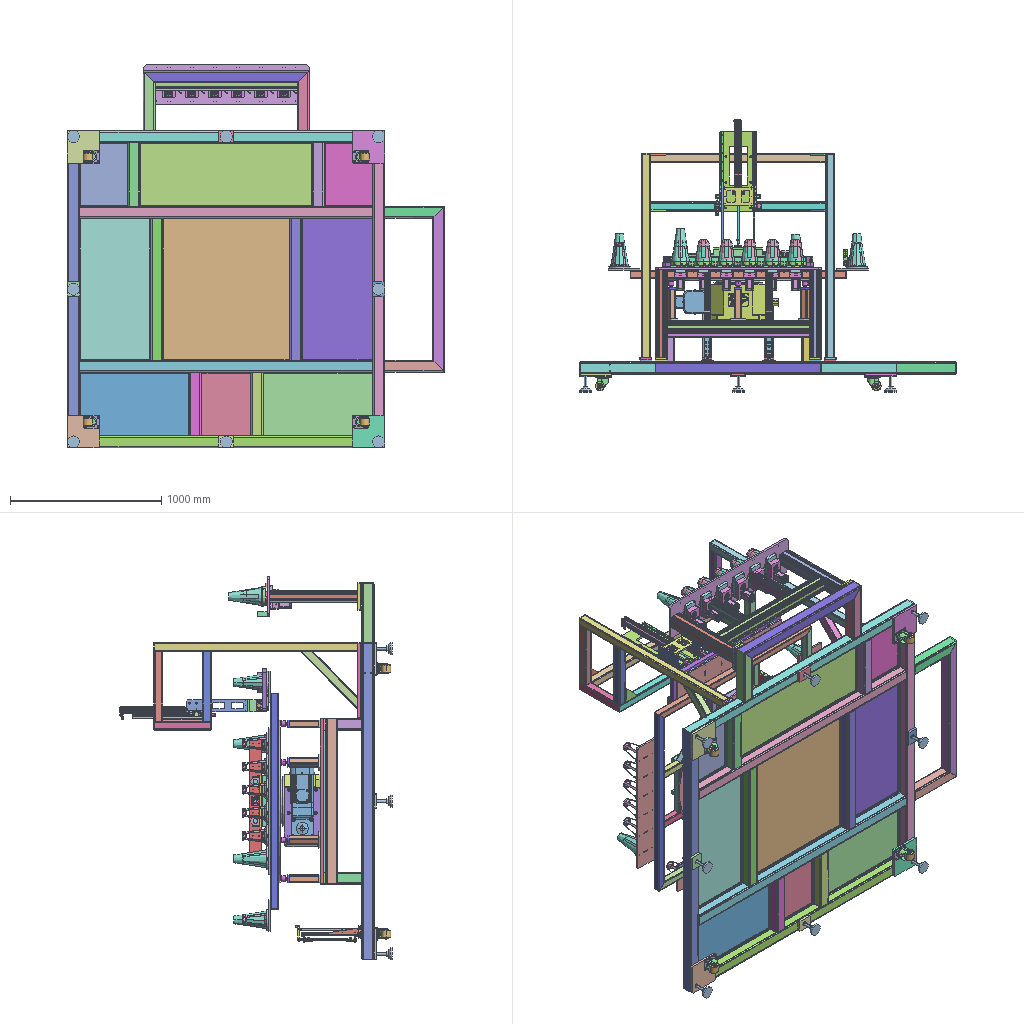Assembly | SolidWorks | 142 different items | 599 placed | box 2495 x 1802 x 2540 mm
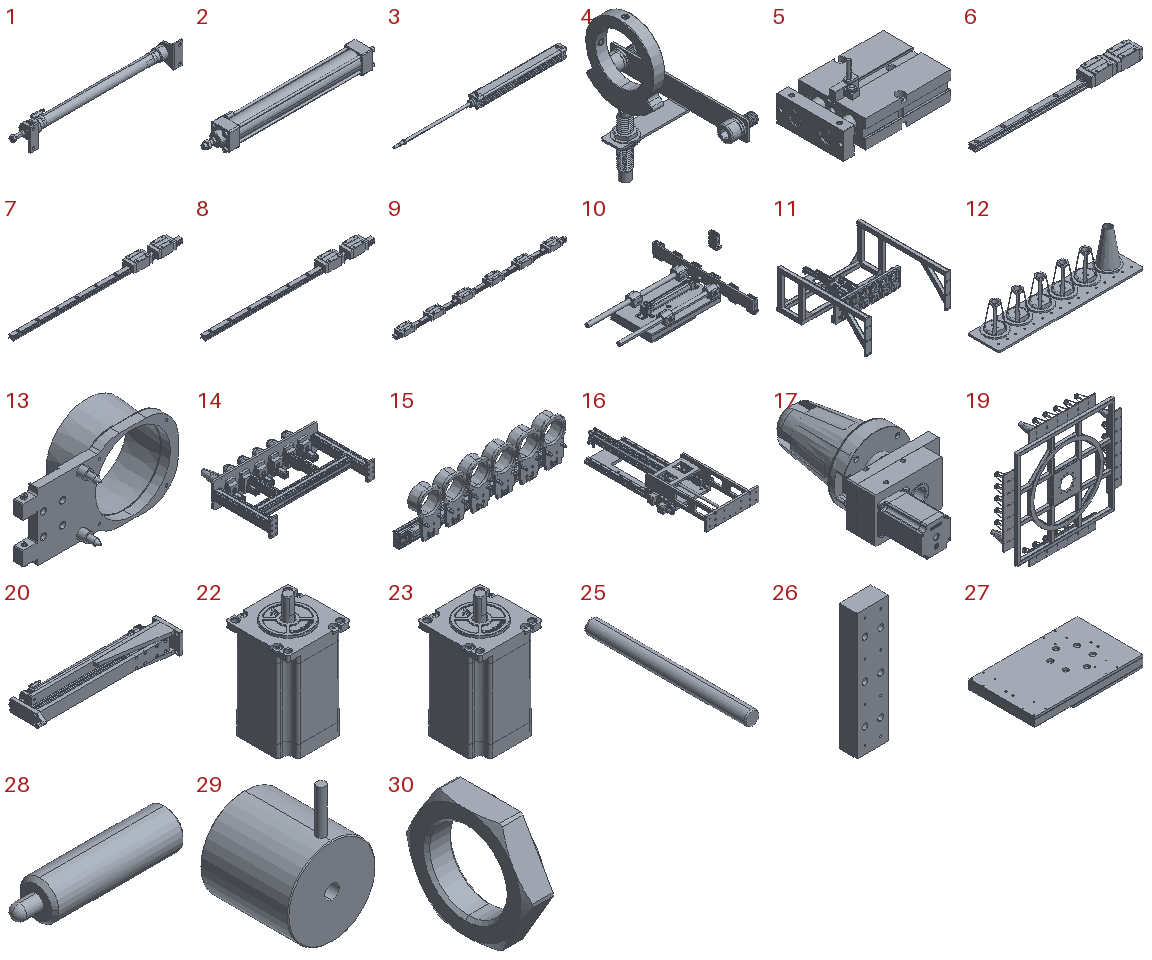Parts list (item | name | quantity | parent item | size | volume | features):
1 | (subassembly) | x2 | in 20 | 392 x 41.5 x 54 mm | 88963 mm3 | -
2 | (subassembly) | x1 | in 10 | 451 x 53.518 x 51.2 mm | 402032 mm3 | -
3 | (subassembly) | x1 | in 16 | 845 x 46.8 x 46.5 mm | 590487 mm3 | -
4 | (subassembly) | x1 | in 24 | 87 x 140.21 x 144 mm | 53103 mm3 | -
5 | (subassembly) | x7 | in 10 | 98 x 62 x 48 mm | 117635 mm3 | -
6 | (subassembly) | x2 | in 20 | 380 x 34 x 28 mm | 139107 mm3 | -
7 | (subassembly) | x1 | in 16 | 520 x 34 x 28 mm | 162854 mm3 | -
8 | (subassembly) | x1 | in 16 | 520 x 34 x 28 mm | 162854 mm3 | -
9 | (subassembly) | x1 | in 15 | 930 x 44 x 30 mm | 645154 mm3 | -
10 | (subassembly) | x1 | in 21 | - | 9355579 mm3 | -
11 | (subassembly) | x1 | in 21 | - | 24248419 mm3 | -
12 | (subassembly) | x4 | in 19 | 975 x 210 x 240 mm | 4305889 mm3 | -
13 | (subassembly) | x6 | in 15 | 257 x 108 x 135 mm | 263904 mm3 | -
14 | (subassembly) | x1 | in 18 | - | 19249167 mm3 | -
15 | (subassembly) | x1 | in 11 | 985 x 114 x 267 mm | 3601226 mm3 | -
16 | (subassembly) | x1 | in 11 | 320 x 857.77 x 130.25 mm | 3607069 mm3 | -
17 | (subassembly) | x6 | in 14 | - | 1851782 mm3 | -
18 | (subassembly) | x1 | in 21 | - | - | -
19 | (subassembly) | x1 | in 21 | - | 27946605 mm3 | -
20 | (subassembly) | x2 | in 21 | 429 x 109.5 x 60 mm | 759599 mm3 | -
21 | (subassembly) | x1 | - | - | - | -
22 | (subassembly) | x6 | in 17 | 56.538 x 56.538 x 106 mm | 169179 mm3 | -
23 | (subassembly) | x6 | in 22 | 56.538 x 56.538 x 106 mm | 169179 mm3 | -
24 | (subassembly) | x1 | in 18 | - | - | -
25 | - | x6 | in 23 | 8 x 92 x 8 mm | 4599 mm3 | features BaseBody 1
26 | - | x1 | in 11 | 80 x 45 x 320 mm | 1113853 mm3 | features BaseBody 1
27 | - | x1 | in 10 | 560 x 340 x 60 mm | 3618040 mm3 | features BaseBody 7
28 | - | x12 | in 13 | 32 x 8 x 8 mm | 1371 mm3 | features BaseBody 1
29 | - | x24 | in 17 | 20 x 20 x 30 mm | 6254 mm3 | features BaseBody 1
30 | - | x4 | in 1 | 7 x 33 x 29 mm | 2695 mm3 | features BaseBody 1
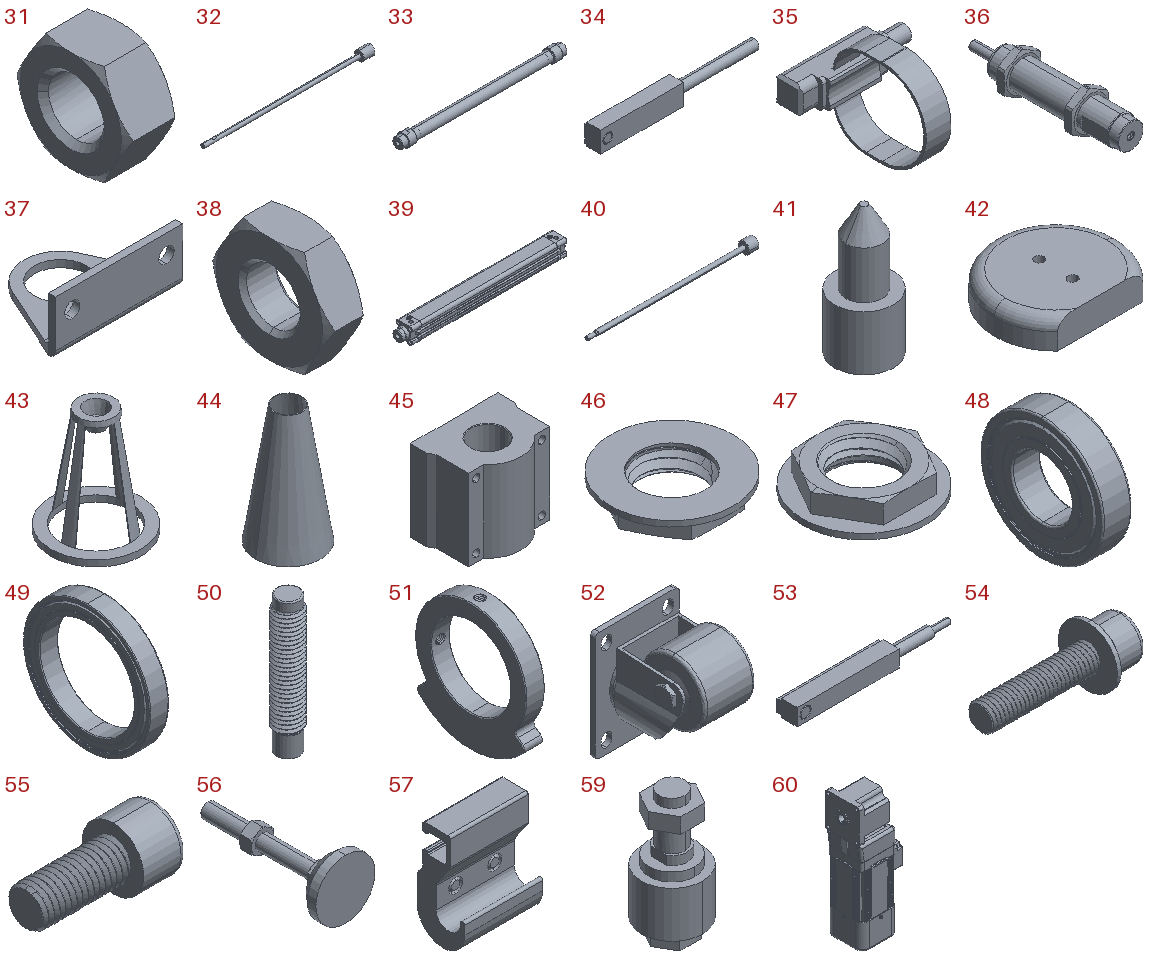31 | - | x2 | in 1 | 6 x 13.856 x 12.001 mm | 526.097 mm3 | features BaseBody 1
32 | - | x2 | in 1 | 339 x 19.5 x 19.5 mm | 22445 mm3 | features BaseBody 1
33 | - | x2 | in 1 | 350 x 27 x 27 mm | 44687 mm3 | features BaseBody 1
34 | - | x1 | in 3 | 48.8 x 5.6 x 6.3 mm | 899.301 mm3 | features BaseBody 1
35 | - | x4 | in 1 | 30 x 30.9 x 22.4 mm | 1513 mm3 | features BaseBody 1
36 | - | x1 | in 16 | 26 x 112.5 x 29.132 mm | 32268 mm3 | features BaseBody 3
37 | - | x4 | in 1 | 54 x 40.5 x 23 mm | 6445 mm3 | features BaseBody 1
38 | - | x1 | in 3 | 6 x 19.63 x 17 mm | 1126 mm3 | features BaseBody 1
39 | - | x1 | in 3 | 466 x 46.5 x 46.5 mm | 520717 mm3 | features BaseBody 1
40 | - | x1 | in 3 | 458 x 31.1 x 31.1 mm | 67743 mm3 | features BaseBody 1
41 | - | x12 | in 13 | 16 x 16 x 35 mm | 4084 mm3 | features BaseBody 1
42 | - | x24 | in 12 | 111 x 95.5 x 25 mm | 213112 mm3 | features BaseBody 1
43 | - | x24 | in 12 | 144 x 144 x 170 mm | 89081 mm3 | features BaseBody 2
44 | - | x5 | in 12, 14 | 120 x 120 x 218 mm | 58583 mm3 | features BaseBody 1
45 | - | x4 | in 10 | 78 x 59.5 x 72 mm | 226738 mm3 | features BaseBody 1
46 | - | x1 | in 4 | 22 x 22 x 4.5 mm | 732.317 mm3 | features BaseBody 1
47 | - | x1 | in 4 | 22 x 22 x 4.5 mm | 732.33 mm3 | features BaseBody 1
48 | - | x6 | in 17 | 17 x 72 x 72 mm | 43583 mm3 | features BaseBody 1
49 | - | x6 | in 17 | 7 x 47 x 47 mm | 4480 mm3 | features BaseBody 1
50 | - | x1 | in 4 | 12 x 12 x 62 mm | 5810 mm3 | features BaseBody 1
51 | - | x1 | in 4 | 12 x 70 x 80 mm | 30669 mm3 | features BaseBody 1
52 | - | x4 | in 18 | 82 x 96 x 111.5 mm | 252248 mm3 | features BaseBody 3
53 | - | x2 | in 2 | 41.8 x 5.7 x 4.4 mm | 661.389 mm3 | features BaseBody 1
54 | - | x4 | in 24 | 53.5 x 22 x 22 mm | 5383 mm3 | features BaseBody 1
55 | - | x4 | in 24 | 40 x 19 x 19 mm | 5409 mm3 | features BaseBody 1
56 | - | x8 | in 18 | 80 x 187 x 80 mm | 168860 mm3 | features BaseBody 2
57 | - | x2 | in 2 | 18 x 12.6 x 23 mm | 2035 mm3 | features BaseBody 1
58 | - | x1 | in 24 | - | - | features BaseBody 1
59 | - | x1 | in 10 | 28 x 28 x 58 mm | 19476 mm3 | features BaseBody 1
60 | - | x1 | in 24 | 220.628 x 166 x 541 mm | 11207085 mm3 | features BaseBody 1
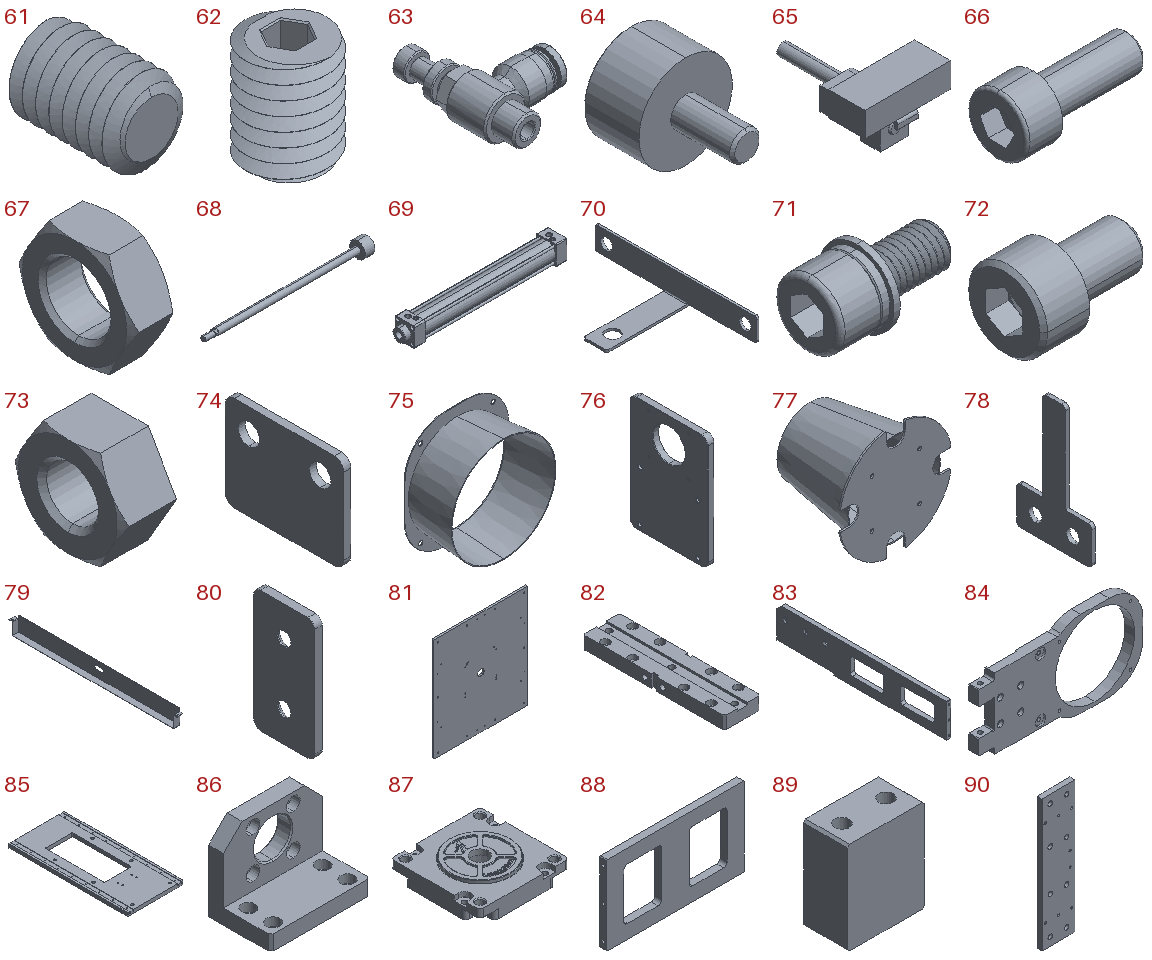61 | - | x1 | in 4 | 6 x 8 x 6 mm | 142.48 mm3 | features BaseBody 1
62 | - | x1 | in 4 | 6 x 6 x 8 mm | 142.472 mm3 | features BaseBody 1
63 | - | x1 | in 16 | 30 x 41.5 x 14 mm | 4765 mm3 | features BaseBody 1
64 | - | x6 | in 18 | 38 x 57 x 38 mm | 31976 mm3 | features BaseBody 1
65 | - | x7 | in 5 | 21 x 26 x 14 mm | 1685 mm3 | features BaseBody 1
66 | - | x4 | in 2 | 22 x 10 x 10 mm | 853.723 mm3 | features BaseBody 1
67 | - | x1 | in 2 | 7 x 19.63 x 17 mm | 1102 mm3 | features BaseBody 1
68 | - | x1 | in 2 | 407.5 x 39.5 x 39.5 mm | 104182 mm3 | features BaseBody 1
69 | - | x1 | in 2 | 408 x 50 x 50 mm | 287943 mm3 | features BaseBody 1
70 | - | x1 | in 4 | 72 x 140.21 x 22 mm | 7925 mm3 | features BaseBody 1
71 | - | x2 | in 4 | 30.5 x 18 x 18 mm | 3479 mm3 | features BaseBody 1
72 | - | x6 | in 13 | 13 x 8.5 x 8.5 mm | 397.23 mm3 | features BaseBody 1
73 | - | x6 | in 18 | 10 x 21.939 x 19 mm | 2287 mm3 | features BaseBody 1
74 | - | x2 | in 16 | 1.5 x 25 x 20 mm | 697.137 mm3 | features BaseBody 1
75 | - | x6 | in 13 | 135 x 61 x 150 mm | 30112 mm3 | features BaseBody 2
76 | - | x1 | in 24 | 20 x 240 x 350 mm | 1488667 mm3 | features BaseBody 1
77 | - | x6 | in 17 | 131.373 x 102 x 131.373 mm | 54164 mm3 | features BaseBody 2
78 | - | x6 | in 17 | 1 x 20 x 34 mm | 323.47 mm3 | features BaseBody 1
79 | - | x1 | in 14 | 35 x 938 x 82 mm | 107925 mm3 | features BaseBody 1
80 | - | x2 | in 15 | 5 x 40 x 80 mm | 14588 mm3 | features BaseBody 1
81 | - | x1 | in 18 | 1000 x 20 x 1100 mm | 21854626 mm3 | features BaseBody 1
82 | - | x2 | in 16 | 35 x 135 x 12 mm | 47871 mm3 | features BaseBody 1
83 | - | x2 | in 16 | 10 x 405 x 80 mm | 250680 mm3 | features BaseBody 1
84 | - | x6 | in 13 | 257 x 15 x 134 mm | 222484 mm3 | features BaseBody 1
85 | - | x1 | in 16 | 245 x 524 x 15 mm | 1411431 mm3 | features BaseBody 1
86 | - | x1 | in 16 | 80 x 50 x 65 mm | 80960 mm3 | features BaseBody 1
87 | - | x6 | in 23 | 56.4 x 56.4 x 13.3 mm | 19484 mm3 | features BaseBody 1
88 | - | x1 | in 16 | 200 x 10 x 115 mm | 146843 mm3 | features BaseBody 1
89 | - | x6 | in 15 | 35 x 20 x 42 mm | 25659 mm3 | features BaseBody 1
90 | - | x1 | in 16 | 80 x 12 x 320 mm | 296552 mm3 | features BaseBody 1
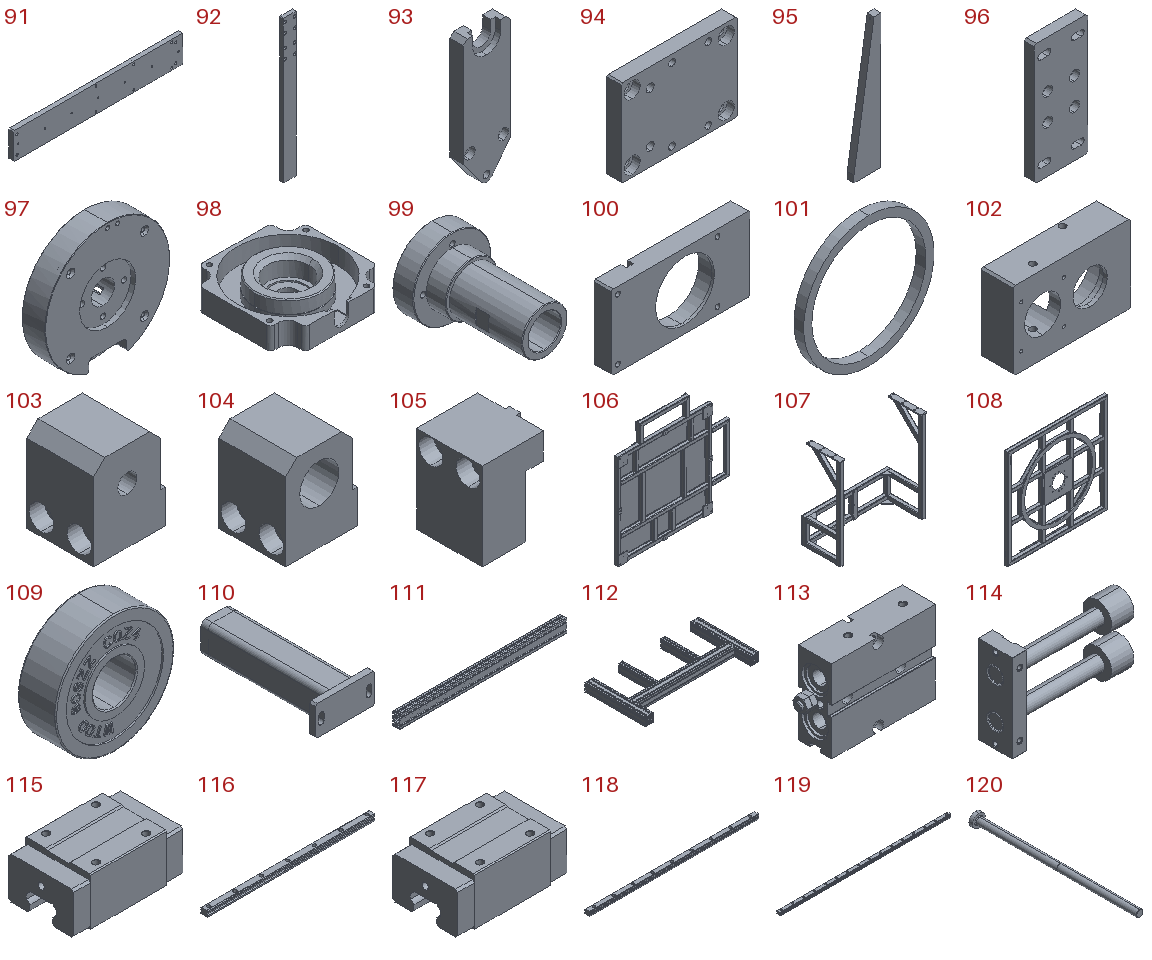91 | - | x2 | in 20 | 380 x 10 x 60 mm | 224318 mm3 | features BaseBody 1
92 | - | x2 | in 20 | 35 x 10 x 380 mm | 129960 mm3 | features BaseBody 1
93 | - | x2 | in 20 | 35 x 10 x 100 mm | 28731 mm3 | features BaseBody 1
94 | - | x2 | in 20 | 80 x 10 x 60 mm | 43027 mm3 | features BaseBody 1
95 | - | x4 | in 20 | 40 x 10 x 200 mm | 51054 mm3 | features BaseBody 1
96 | - | x2 | in 14 | 80 x 15 x 180 mm | 198624 mm3 | features BaseBody 1
97 | - | x6 | in 17 | 134 x 25 x 134 mm | 280686 mm3 | features BaseBody 1
98 | - | x6 | in 23 | - | - | features RefSurface 4, BaseBody 1
99 | - | x6 | in 17 | 60 x 87 x 60 mm | 74210 mm3 | features BaseBody 1
100 | - | x6 | in 17 | 160 x 20 x 86 mm | 181258 mm3 | features BaseBody 1
101 | - | x12 | in 17 | 40 x 3 x 40 mm | 883.573 mm3 | features BaseBody 1
102 | - | x6 | in 17 | 130 x 35.485 x 86 mm | 236354 mm3 | features BaseBody 1
103 | - | x1 | in 16 | 34 x 30 x 40 mm | 31581 mm3 | features BaseBody 1
104 | - | x1 | in 16 | 34 x 30 x 40 mm | 26067 mm3 | features BaseBody 1
105 | - | x2 | in 16 | 30 x 30 x 40 mm | 24257 mm3 | features BaseBody 1
106 | - | x1 | in 18 | 2495 x 350 x 2495 mm | 50017538 mm3 | features BaseBody 53
107 | - | x1 | in 11 | 1300 x 580 x 1365 mm | 9754704 mm3 | features BaseBody 24
108 | - | x1 | in 19 | 1430 x 67 x 1430 mm | 10727626 mm3 | features BaseBody 26
109 | - | x6 | in 23 | 22 x 7 x 22 mm | 2214 mm3 | features BaseBody 1
110 | - | x6 | in 18 | 100 x 217 x 50 mm | 210593 mm3 | features BaseBody 3
111 | - | x1 | in 15 | 975 x 40 x 80 mm | 1189517 mm3 | features BaseBody 1
112 | - | x1 | in 14 | 1100 x 583 x 80 mm | 4144887 mm3 | features BaseBody 5
113 | - | x7 | in 5 | 88 x 25 x 62 mm | 82875 mm3 | features BaseBody 1
114 | - | x7 | in 5 | 86.6 x 24 x 61 mm | 33075 mm3 | features BaseBody 1
115 | - | x4 | in 6 | 56.9 x 34 x 24.8 mm | 37620 mm3 | features BaseBody 1
116 | - | x2 | in 6 | 380 x 15 x 13 mm | 63866 mm3 | features BaseBody 1
117 | - | x4 | in 7, 8 | 56.9 x 34 x 24.8 mm | 37620 mm3 | features BaseBody 1
118 | - | x2 | in 7, 8 | 520 x 15 x 13 mm | 87614 mm3 | features BaseBody 1
119 | - | x1 | in 9 | 930 x 20 x 16.5 mm | 262236 mm3 | features BaseBody 1
120 | - | x48 | in 23 | - | - | features BaseBody 1, RefSurface 1
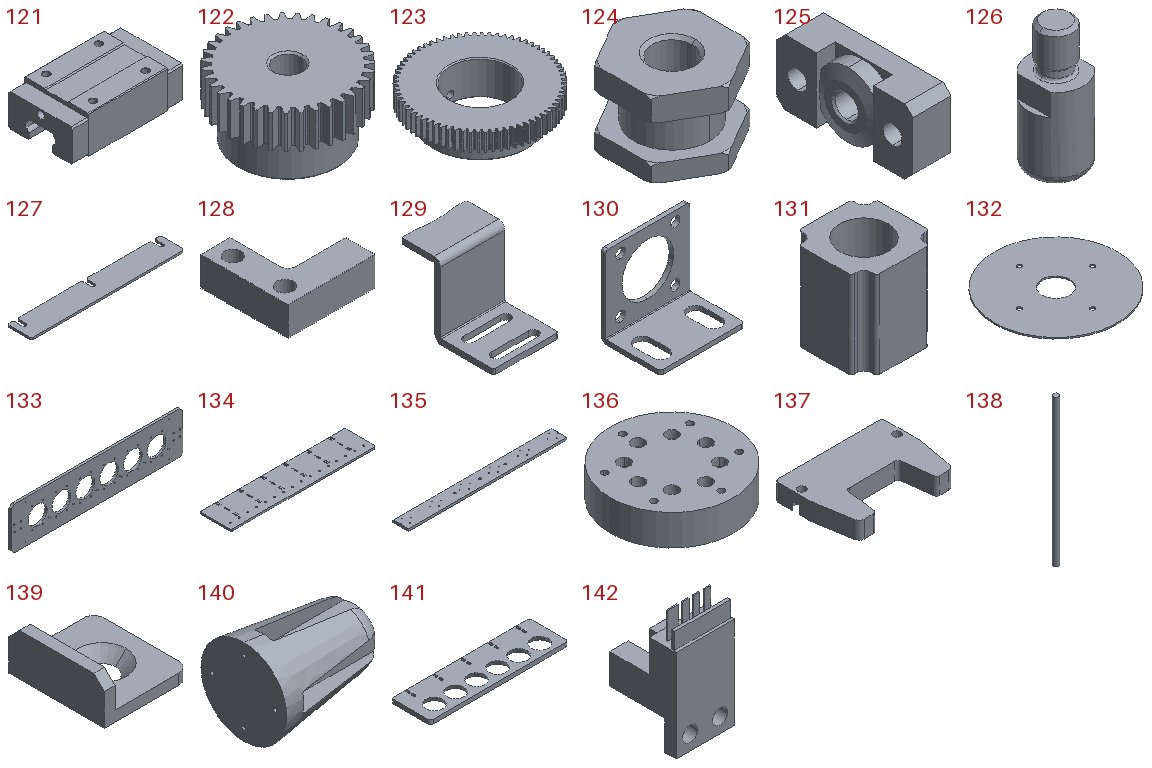121 | - | x6 | in 9 | 75.6 x 44 x 25.4 mm | 63820 mm3 | features BaseBody 1
122 | - | x6 | in 17 | 36.989 x 36.955 x 20 mm | 15313 mm3 | features BaseBody 1
123 | - | x6 | in 17 | 71.959 x 72 x 20 mm | 43377 mm3 | features BaseBody 1
124 | - | x2 | in 20 | 17 x 19.6 x 13 mm | 2052 mm3 | features BaseBody 1
125 | - | x1 | in 16 | 16 x 50 x 24 mm | 13355 mm3 | features BaseBody 2
126 | - | x2 | in 20 | 10 x 10 x 23 mm | 1337 mm3 | features BaseBody 1
127 | - | x2 | in 11 | 380 x 60 x 5 mm | 109700 mm3 | features BaseBody 1
128 | - | x1 | in 14 | 30 x 30 x 10 mm | 4491 mm3 | features BaseBody 1
129 | - | x6 | in 14 | 35 x 50 x 40 mm | 8107 mm3 | features BaseBody 1
130 | - | x2 | in 10 | 57 x 40 x 55 mm | 10916 mm3 | features BaseBody 1
131 | - | x6 | in 23 | 56.4 x 56.4 x 63 mm | 119307 mm3 | features BaseBody 1
132 | - | x6 | in 17 | 134 x 134 x 1.5 mm | 19985 mm3 | features BaseBody 1
133 | - | x1 | in 14 | 1100 x 15 x 270 mm | 3383185 mm3 | features BaseBody 1
134 | - | x4 | in 12 | 975 x 210 x 12 mm | 2426074 mm3 | features BaseBody 1
135 | - | x1 | in 10 | 824 x 80 x 12 mm | 783419 mm3 | features BaseBody 1
136 | - | x1 | in 10 | 200 x 200 x 50 mm | 1483994 mm3 | features BaseBody 1
137 | - | x7 | in 10 | 62 x 45 x 10 mm | 19803 mm3 | features BaseBody 1
138 | - | x2 | in 10 | 30 x 30 x 820 mm | 578882 mm3 | features BaseBody 1
139 | - | x48 | in 12 | 16 x 18 x 8 mm | 697.494 mm3 | features BaseBody 1
140 | - | x6 | in 17 | 145 x 109 x 109 mm | 700128 mm3 | features BaseBody 1
141 | - | x1 | in 11 | 1000 x 282 x 30 mm | 5952206 mm3 | features BaseBody 1
142 | - | x6 | in 17 | 13.6 x 15.5 x 27.7 mm | 2033 mm3 | features BaseBody 1